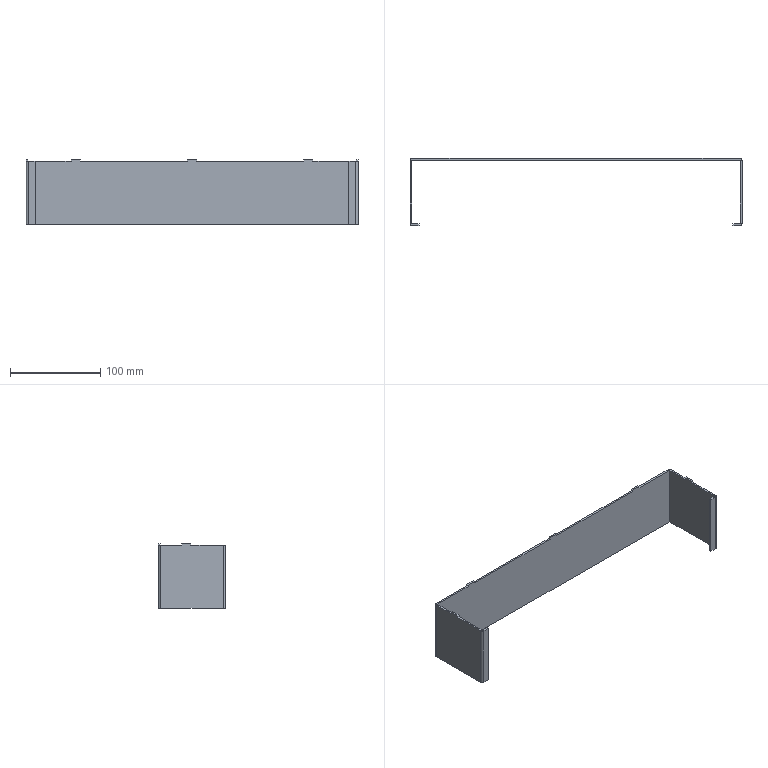Part | STEP file | xzz-004 | 1 solid | 42 faces | box 368 x 74.5 x 72 mm | volume 73899 mm3 | plane 34 | cylinder 8 | commonest cylinder face diameters 1 x4 5 x4
STEP:
#1=CARTESIAN_POINT('',(157.,14.,70.));
#2=VERTEX_POINT('',#1);
#3=CARTESIAN_POINT('',(204.5,14.,70.));
#4=VERTEX_POINT('',#3);
#5=CARTESIAN_POINT('',(-161.,14.,70.));
#6=DIRECTION('',(1.,0.,0.));
#7=VECTOR('',#6,1000.);
#8=LINE('',#5,#7);
#9=EDGE_CURVE('',#2,#4,#8,.T.);
#10=ORIENTED_EDGE('',*,*,#9,.T.);
#11=CARTESIAN_POINT('',(204.5,14.,0.));
#12=VERTEX_POINT('',#11);
#13=CARTESIAN_POINT('',(204.5,14.,70.));
#14=DIRECTION('',(0.,0.,-1.));
#15=VECTOR('',#14,1000.);
#16=LINE('',#13,#15);
#17=EDGE_CURVE('',#4,#12,#16,.T.);
#18=ORIENTED_EDGE('',*,*,#17,.T.);
#19=CARTESIAN_POINT('',(-158.5,14.,0.));
#20=VERTEX_POINT('',#19);
#21=CARTESIAN_POINT('',(-161.,14.,0.));
#22=DIRECTION('',(-1.,0.,0.));
#23=VECTOR('',#22,1000.);
#24=LINE('',#21,#23);
#25=EDGE_CURVE('',#12,#20,#24,.T.);
#26=ORIENTED_EDGE('',*,*,#25,.T.);
#27=CARTESIAN_POINT('',(-158.5,14.,70.));
#28=VERTEX_POINT('',#27);
#29=CARTESIAN_POINT('',(-158.5,14.,70.));
#30=DIRECTION('',(0.,0.,1.));
#31=VECTOR('',#30,1000.);
#32=LINE('',#29,#31);
#33=EDGE_CURVE('',#20,#28,#32,.T.);
#34=ORIENTED_EDGE('',*,*,#33,.T.);
#35=CARTESIAN_POINT('',(-111.,14.,70.));
#36=VERTEX_POINT('',#35);
#37=CARTESIAN_POINT('',(-161.,14.,70.));
#38=DIRECTION('',(1.,0.,0.));
#39=VECTOR('',#38,1000.);
#40=LINE('',#37,#39);
#41=EDGE_CURVE('',#28,#36,#40,.T.);
#42=ORIENTED_EDGE('',*,*,#41,.T.);
#43=CARTESIAN_POINT('',(-111.,14.,72.));
#44=VERTEX_POINT('',#43);
#45=CARTESIAN_POINT('',(-111.,14.,70.));
#46=DIRECTION('',(0.,0.,1.));
#47=VECTOR('',#46,1000.);
#48=LINE('',#45,#47);
#49=EDGE_CURVE('',#36,#44,#48,.T.);
#50=ORIENTED_EDGE('',*,*,#49,.T.);
#51=CARTESIAN_POINT('',(-101.,14.,72.));
#52=VERTEX_POINT('',#51);
#53=CARTESIAN_POINT('',(-161.,14.,72.));
#54=DIRECTION('',(1.,0.,0.));
#55=VECTOR('',#54,1000.);
#56=LINE('',#53,#55);
#57=EDGE_CURVE('',#44,#52,#56,.T.);
#58=ORIENTED_EDGE('',*,*,#57,.T.);
#59=CARTESIAN_POINT('',(-101.,14.,70.));
#60=VERTEX_POINT('',#59);
#61=CARTESIAN_POINT('',(-101.,14.,70.));
#62=DIRECTION('',(0.,0.,-1.));
#63=VECTOR('',#62,1000.);
#64=LINE('',#61,#63);
#65=EDGE_CURVE('',#52,#60,#64,.T.);
#66=ORIENTED_EDGE('',*,*,#65,.T.);
#67=CARTESIAN_POINT('',(18.,14.,70.));
#68=VERTEX_POINT('',#67);
#69=CARTESIAN_POINT('',(-161.,14.,70.));
#70=DIRECTION('',(1.,0.,0.));
#71=VECTOR('',#70,1000.);
#72=LINE('',#69,#71);
#73=EDGE_CURVE('',#60,#68,#72,.T.);
#74=ORIENTED_EDGE('',*,*,#73,.T.);
#75=CARTESIAN_POINT('',(18.,14.,72.));
#76=VERTEX_POINT('',#75);
#77=CARTESIAN_POINT('',(18.,14.,70.));
#78=DIRECTION('',(0.,0.,1.));
#79=VECTOR('',#78,1000.);
#80=LINE('',#77,#79);
#81=EDGE_CURVE('',#68,#76,#80,.T.);
#82=ORIENTED_EDGE('',*,*,#81,.T.);
#83=CARTESIAN_POINT('',(28.,14.,72.));
#84=VERTEX_POINT('',#83);
#85=CARTESIAN_POINT('',(-161.,14.,72.));
#86=DIRECTION('',(1.,0.,0.));
#87=VECTOR('',#86,1000.);
#88=LINE('',#85,#87);
#89=EDGE_CURVE('',#76,#84,#88,.T.);
#90=ORIENTED_EDGE('',*,*,#89,.T.);
#91=CARTESIAN_POINT('',(28.,14.,70.));
#92=VERTEX_POINT('',#91);
#93=CARTESIAN_POINT('',(28.,14.,70.));
#94=DIRECTION('',(0.,0.,-1.));
#95=VECTOR('',#94,1000.);
#96=LINE('',#93,#95);
#97=EDGE_CURVE('',#84,#92,#96,.T.);
#98=ORIENTED_EDGE('',*,*,#97,.T.);
#99=CARTESIAN_POINT('',(147.,14.,70.));
#100=VERTEX_POINT('',#99);
#101=CARTESIAN_POINT('',(-161.,14.,70.));
#102=DIRECTION('',(1.,0.,0.));
#103=VECTOR('',#102,1000.);
#104=LINE('',#101,#103);
#105=EDGE_CURVE('',#92,#100,#104,.T.);
#106=ORIENTED_EDGE('',*,*,#105,.T.);
#107=CARTESIAN_POINT('',(147.,14.,72.));
#108=VERTEX_POINT('',#107);
#109=CARTESIAN_POINT('',(147.,14.,70.));
#110=DIRECTION('',(0.,0.,1.));
#111=VECTOR('',#110,1000.);
#112=LINE('',#109,#111);
#113=EDGE_CURVE('',#100,#108,#112,.T.);
#114=ORIENTED_EDGE('',*,*,#113,.T.);
#115=CARTESIAN_POINT('',(157.,14.,72.));
#116=VERTEX_POINT('',#115);
#117=CARTESIAN_POINT('',(-161.,14.,72.));
#118=DIRECTION('',(1.,0.,0.));
#119=VECTOR('',#118,1000.);
#120=LINE('',#117,#119);
#121=EDGE_CURVE('',#108,#116,#120,.T.);
#122=ORIENTED_EDGE('',*,*,#121,.T.);
#123=CARTESIAN_POINT('',(157.,14.,70.));
#124=DIRECTION('',(0.,0.,-1.));
#125=VECTOR('',#124,1000.);
#126=LINE('',#123,#125);
#127=EDGE_CURVE('',#116,#2,#126,.T.);
#128=ORIENTED_EDGE('',*,*,#127,.T.);
#129=EDGE_LOOP('',(#10,#18,#26,#34,#42,#50,#58,#66,#74,#82,#90,#98,#106,#114,#122,#128));
#130=FACE_OUTER_BOUND('',#129,.T.);
#131=CARTESIAN_POINT('',(-161.,14.,70.));
#132=DIRECTION('',(0.,1.,0.));
#133=DIRECTION('',(0.,0.,1.));
#134=AXIS2_PLACEMENT_3D('',#131,#132,#133);
#135=PLANE('',#134);
#136=ADVANCED_FACE('',(#130),#135,.T.);
#137=CARTESIAN_POINT('',(207.,11.5,70.));
#138=VERTEX_POINT('',#137);
#139=CARTESIAN_POINT('',(204.5,11.5,70.));
#140=DIRECTION('',(0.,0.,-1.));
#141=DIRECTION('',(-1.,0.,0.));
#142=AXIS2_PLACEMENT_3D('',#139,#140,#141);
#143=CIRCLE('',#142,2.5);
#144=EDGE_CURVE('',#4,#138,#143,.T.);
#145=ORIENTED_EDGE('',*,*,#144,.T.);
#146=CARTESIAN_POINT('',(207.,11.5,0.));
#147=VERTEX_POINT('',#146);
#148=CARTESIAN_POINT('',(207.,11.5,70.));
#149=DIRECTION('',(0.,0.,-1.));
#150=VECTOR('',#149,1000.);
#151=LINE('',#148,#150);
#152=EDGE_CURVE('',#138,#147,#151,.T.);
#153=ORIENTED_EDGE('',*,*,#152,.T.);
#154=CARTESIAN_POINT('',(204.5,11.5,0.));
#155=DIRECTION('',(0.,0.,1.));
#156=DIRECTION('',(-1.,0.,0.));
#157=AXIS2_PLACEMENT_3D('',#154,#155,#156);
#158=CIRCLE('',#157,2.5);
#159=EDGE_CURVE('',#147,#12,#158,.T.);
#160=ORIENTED_EDGE('',*,*,#159,.T.);
#161=ORIENTED_EDGE('',*,*,#17,.F.);
#162=EDGE_LOOP('',(#145,#153,#160,#161));
#163=FACE_OUTER_BOUND('',#162,.T.);
#164=CARTESIAN_POINT('',(204.5,11.5,70.));
#165=DIRECTION('',(0.,0.,-1.));
#166=DIRECTION('',(-1.,0.,0.));
#167=AXIS2_PLACEMENT_3D('',#164,#165,#166);
#168=CYLINDRICAL_SURFACE('',#167,2.5);
#169=ADVANCED_FACE('',(#163),#168,.T.);
#170=CARTESIAN_POINT('',(157.,12.,70.));
#171=VERTEX_POINT('',#170);
#172=CARTESIAN_POINT('',(204.5,12.,70.));
#173=VERTEX_POINT('',#172);
#174=CARTESIAN_POINT('',(-159.,12.,70.));
#175=DIRECTION('',(1.,0.,0.));
#176=VECTOR('',#175,1000.);
#177=LINE('',#174,#176);
#178=EDGE_CURVE('',#171,#173,#177,.T.);
#179=ORIENTED_EDGE('',*,*,#178,.T.);
#180=CARTESIAN_POINT('',(205.,11.5,70.));
#181=VERTEX_POINT('',#180);
#182=CARTESIAN_POINT('',(204.5,11.5,70.));
#183=DIRECTION('',(0.,0.,-1.));
#184=DIRECTION('',(-1.,0.,0.));
#185=AXIS2_PLACEMENT_3D('',#182,#183,#184);
#186=CIRCLE('',#185,0.5);
#187=EDGE_CURVE('',#173,#181,#186,.T.);
#188=ORIENTED_EDGE('',*,*,#187,.T.);
#189=CARTESIAN_POINT('',(205.,-12.,70.));
#190=VERTEX_POINT('',#189);
#191=CARTESIAN_POINT('',(205.,12.,70.));
#192=DIRECTION('',(0.,-1.,0.));
#193=VECTOR('',#192,1000.);
#194=LINE('',#191,#193);
#195=EDGE_CURVE('',#181,#190,#194,.T.);
#196=ORIENTED_EDGE('',*,*,#195,.T.);
#197=CARTESIAN_POINT('',(207.,-12.,70.));
#198=VERTEX_POINT('',#197);
#199=CARTESIAN_POINT('',(205.,-12.,70.));
#200=DIRECTION('',(1.,0.,0.));
#201=VECTOR('',#200,1000.);
#202=LINE('',#199,#201);
#203=EDGE_CURVE('',#190,#198,#202,.T.);
#204=ORIENTED_EDGE('',*,*,#203,.T.);
#205=CARTESIAN_POINT('',(207.,14.,70.));
#206=DIRECTION('',(0.,-1.,0.));
#207=VECTOR('',#206,1000.);
#208=LINE('',#205,#207);
#209=EDGE_CURVE('',#138,#198,#208,.T.);
#210=ORIENTED_EDGE('',*,*,#209,.F.);
#211=ORIENTED_EDGE('',*,*,#144,.F.);
#212=ORIENTED_EDGE('',*,*,#9,.F.);
#213=CARTESIAN_POINT('',(157.,11.5,70.));
#214=DIRECTION('',(0.,-1.,0.));
#215=VECTOR('',#214,1000.);
#216=LINE('',#213,#215);
#217=EDGE_CURVE('',#2,#171,#216,.T.);
#218=ORIENTED_EDGE('',*,*,#217,.T.);
#219=EDGE_LOOP('',(#179,#188,#196,#204,#210,#211,#212,#218));
#220=FACE_OUTER_BOUND('',#219,.T.);
#221=CARTESIAN_POINT('',(-159.,11.5,70.));
#222=DIRECTION('',(0.,0.,1.));
#223=DIRECTION('',(1.,0.,0.));
#224=AXIS2_PLACEMENT_3D('',#221,#222,#223);
#225=PLANE('',#224);
#226=ADVANCED_FACE('',(#220),#225,.T.);
#227=ORIENTED_EDGE('',*,*,#127,.F.);
#228=CARTESIAN_POINT('',(157.,12.,72.));
#229=VERTEX_POINT('',#228);
#230=CARTESIAN_POINT('',(157.,14.,72.));
#231=DIRECTION('',(0.,1.,0.));
#232=VECTOR('',#231,1000.);
#233=LINE('',#230,#232);
#234=EDGE_CURVE('',#229,#116,#233,.T.);
#235=ORIENTED_EDGE('',*,*,#234,.F.);
#236=CARTESIAN_POINT('',(157.,12.,72.));
#237=DIRECTION('',(0.,0.,1.));
#238=VECTOR('',#237,1000.);
#239=LINE('',#236,#238);
#240=EDGE_CURVE('',#171,#229,#239,.T.);
#241=ORIENTED_EDGE('',*,*,#240,.F.);
#242=ORIENTED_EDGE('',*,*,#217,.F.);
#243=EDGE_LOOP('',(#227,#235,#241,#242));
#244=FACE_OUTER_BOUND('',#243,.T.);
#245=CARTESIAN_POINT('',(157.,14.,72.));
#246=DIRECTION('',(-1.,0.,0.));
#247=DIRECTION('',(0.,0.,1.));
#248=AXIS2_PLACEMENT_3D('',#245,#246,#247);
#249=PLANE('',#248);
#250=ADVANCED_FACE('',(#244),#249,.F.);
#251=ORIENTED_EDGE('',*,*,#234,.T.);
#252=ORIENTED_EDGE('',*,*,#121,.F.);
#253=CARTESIAN_POINT('',(147.,12.,72.));
#254=VERTEX_POINT('',#253);
#255=CARTESIAN_POINT('',(147.,0.,72.));
#256=DIRECTION('',(0.,-1.,0.));
#257=VECTOR('',#256,1000.);
#258=LINE('',#255,#257);
#259=EDGE_CURVE('',#108,#254,#258,.T.);
#260=ORIENTED_EDGE('',*,*,#259,.T.);
#261=CARTESIAN_POINT('',(0.,12.,72.));
#262=DIRECTION('',(1.,0.,0.));
#263=VECTOR('',#262,1000.);
#264=LINE('',#261,#263);
#265=EDGE_CURVE('',#254,#229,#264,.T.);
#266=ORIENTED_EDGE('',*,*,#265,.T.);
#267=EDGE_LOOP('',(#251,#252,#260,#266));
#268=FACE_OUTER_BOUND('',#267,.T.);
#269=CARTESIAN_POINT('',(0.,0.,72.));
#270=DIRECTION('',(0.,0.,1.));
#271=DIRECTION('',(1.,0.,0.));
#272=AXIS2_PLACEMENT_3D('',#269,#270,#271);
#273=PLANE('',#272);
#274=ADVANCED_FACE('',(#268),#273,.T.);
#275=CARTESIAN_POINT('',(147.,12.,70.));
#276=VERTEX_POINT('',#275);
#277=CARTESIAN_POINT('',(147.,12.,72.));
#278=DIRECTION('',(0.,0.,-1.));
#279=VECTOR('',#278,1000.);
#280=LINE('',#277,#279);
#281=EDGE_CURVE('',#254,#276,#280,.T.);
#282=ORIENTED_EDGE('',*,*,#281,.F.);
#283=ORIENTED_EDGE('',*,*,#259,.F.);
#284=ORIENTED_EDGE('',*,*,#113,.F.);
#285=CARTESIAN_POINT('',(147.,14.,70.));
#286=DIRECTION('',(0.,1.,0.));
#287=VECTOR('',#286,1000.);
#288=LINE('',#285,#287);
#289=EDGE_CURVE('',#276,#100,#288,.T.);
#290=ORIENTED_EDGE('',*,*,#289,.F.);
#291=EDGE_LOOP('',(#282,#283,#284,#290));
#292=FACE_OUTER_BOUND('',#291,.T.);
#293=CARTESIAN_POINT('',(147.,14.,72.));
#294=DIRECTION('',(1.,0.,0.));
#295=DIRECTION('',(0.,0.,-1.));
#296=AXIS2_PLACEMENT_3D('',#293,#294,#295);
#297=PLANE('',#296);
#298=ADVANCED_FACE('',(#292),#297,.F.);
#299=ORIENTED_EDGE('',*,*,#105,.F.);
#300=CARTESIAN_POINT('',(28.,12.,70.));
#301=VERTEX_POINT('',#300);
#302=CARTESIAN_POINT('',(28.,11.5,70.));
#303=DIRECTION('',(0.,-1.,0.));
#304=VECTOR('',#303,1000.);
#305=LINE('',#302,#304);
#306=EDGE_CURVE('',#92,#301,#305,.T.);
#307=ORIENTED_EDGE('',*,*,#306,.T.);
#308=CARTESIAN_POINT('',(-159.,12.,70.));
#309=DIRECTION('',(1.,0.,0.));
#310=VECTOR('',#309,1000.);
#311=LINE('',#308,#310);
#312=EDGE_CURVE('',#301,#276,#311,.T.);
#313=ORIENTED_EDGE('',*,*,#312,.T.);
#314=ORIENTED_EDGE('',*,*,#289,.T.);
#315=EDGE_LOOP('',(#299,#307,#313,#314));
#316=FACE_OUTER_BOUND('',#315,.T.);
#317=CARTESIAN_POINT('',(-159.,11.5,70.));
#318=DIRECTION('',(0.,0.,1.));
#319=DIRECTION('',(1.,0.,0.));
#320=AXIS2_PLACEMENT_3D('',#317,#318,#319);
#321=PLANE('',#320);
#322=ADVANCED_FACE('',(#316),#321,.T.);
#323=ORIENTED_EDGE('',*,*,#97,.F.);
#324=CARTESIAN_POINT('',(28.,12.,72.));
#325=VERTEX_POINT('',#324);
#326=CARTESIAN_POINT('',(28.,14.,72.));
#327=DIRECTION('',(0.,1.,0.));
#328=VECTOR('',#327,1000.);
#329=LINE('',#326,#328);
#330=EDGE_CURVE('',#325,#84,#329,.T.);
#331=ORIENTED_EDGE('',*,*,#330,.F.);
#332=CARTESIAN_POINT('',(28.,12.,72.));
#333=DIRECTION('',(0.,0.,1.));
#334=VECTOR('',#333,1000.);
#335=LINE('',#332,#334);
#336=EDGE_CURVE('',#301,#325,#335,.T.);
#337=ORIENTED_EDGE('',*,*,#336,.F.);
#338=ORIENTED_EDGE('',*,*,#306,.F.);
#339=EDGE_LOOP('',(#323,#331,#337,#338));
#340=FACE_OUTER_BOUND('',#339,.T.);
#341=CARTESIAN_POINT('',(28.,14.,72.));
#342=DIRECTION('',(-1.,0.,0.));
#343=DIRECTION('',(0.,0.,1.));
#344=AXIS2_PLACEMENT_3D('',#341,#342,#343);
#345=PLANE('',#344);
#346=ADVANCED_FACE('',(#340),#345,.F.);
#347=ORIENTED_EDGE('',*,*,#330,.T.);
#348=ORIENTED_EDGE('',*,*,#89,.F.);
#349=CARTESIAN_POINT('',(18.,12.,72.));
#350=VERTEX_POINT('',#349);
#351=CARTESIAN_POINT('',(18.,0.,72.));
#352=DIRECTION('',(0.,-1.,0.));
#353=VECTOR('',#352,1000.);
#354=LINE('',#351,#353);
#355=EDGE_CURVE('',#76,#350,#354,.T.);
#356=ORIENTED_EDGE('',*,*,#355,.T.);
#357=CARTESIAN_POINT('',(0.,12.,72.));
#358=DIRECTION('',(1.,0.,0.));
#359=VECTOR('',#358,1000.);
#360=LINE('',#357,#359);
#361=EDGE_CURVE('',#350,#325,#360,.T.);
#362=ORIENTED_EDGE('',*,*,#361,.T.);
#363=EDGE_LOOP('',(#347,#348,#356,#362));
#364=FACE_OUTER_BOUND('',#363,.T.);
#365=CARTESIAN_POINT('',(0.,0.,72.));
#366=DIRECTION('',(0.,0.,1.));
#367=DIRECTION('',(1.,0.,0.));
#368=AXIS2_PLACEMENT_3D('',#365,#366,#367);
#369=PLANE('',#368);
#370=ADVANCED_FACE('',(#364),#369,.T.);
#371=CARTESIAN_POINT('',(18.,12.,70.));
#372=VERTEX_POINT('',#371);
#373=CARTESIAN_POINT('',(18.,12.,72.));
#374=DIRECTION('',(0.,0.,-1.));
#375=VECTOR('',#374,1000.);
#376=LINE('',#373,#375);
#377=EDGE_CURVE('',#350,#372,#376,.T.);
#378=ORIENTED_EDGE('',*,*,#377,.F.);
#379=ORIENTED_EDGE('',*,*,#355,.F.);
#380=ORIENTED_EDGE('',*,*,#81,.F.);
#381=CARTESIAN_POINT('',(18.,14.,70.));
#382=DIRECTION('',(0.,1.,0.));
#383=VECTOR('',#382,1000.);
#384=LINE('',#381,#383);
#385=EDGE_CURVE('',#372,#68,#384,.T.);
#386=ORIENTED_EDGE('',*,*,#385,.F.);
#387=EDGE_LOOP('',(#378,#379,#380,#386));
#388=FACE_OUTER_BOUND('',#387,.T.);
#389=CARTESIAN_POINT('',(18.,14.,72.));
#390=DIRECTION('',(1.,0.,0.));
#391=DIRECTION('',(0.,0.,-1.));
#392=AXIS2_PLACEMENT_3D('',#389,#390,#391);
#393=PLANE('',#392);
#394=ADVANCED_FACE('',(#388),#393,.F.);
#395=ORIENTED_EDGE('',*,*,#73,.F.);
#396=CARTESIAN_POINT('',(-101.,12.,70.));
#397=VERTEX_POINT('',#396);
#398=CARTESIAN_POINT('',(-101.,11.5,70.));
#399=DIRECTION('',(0.,-1.,0.));
#400=VECTOR('',#399,1000.);
#401=LINE('',#398,#400);
#402=EDGE_CURVE('',#60,#397,#401,.T.);
#403=ORIENTED_EDGE('',*,*,#402,.T.);
#404=CARTESIAN_POINT('',(-159.,12.,70.));
#405=DIRECTION('',(1.,0.,0.));
#406=VECTOR('',#405,1000.);
#407=LINE('',#404,#406);
#408=EDGE_CURVE('',#397,#372,#407,.T.);
#409=ORIENTED_EDGE('',*,*,#408,.T.);
#410=ORIENTED_EDGE('',*,*,#385,.T.);
#411=EDGE_LOOP('',(#395,#403,#409,#410));
#412=FACE_OUTER_BOUND('',#411,.T.);
#413=CARTESIAN_POINT('',(-159.,11.5,70.));
#414=DIRECTION('',(0.,0.,1.));
#415=DIRECTION('',(1.,0.,0.));
#416=AXIS2_PLACEMENT_3D('',#413,#414,#415);
#417=PLANE('',#416);
#418=ADVANCED_FACE('',(#412),#417,.T.);
#419=ORIENTED_EDGE('',*,*,#65,.F.);
#420=CARTESIAN_POINT('',(-101.,12.,72.));
#421=VERTEX_POINT('',#420);
#422=CARTESIAN_POINT('',(-101.,14.,72.));
#423=DIRECTION('',(0.,1.,0.));
#424=VECTOR('',#423,1000.);
#425=LINE('',#422,#424);
#426=EDGE_CURVE('',#421,#52,#425,.T.);
#427=ORIENTED_EDGE('',*,*,#426,.F.);
#428=CARTESIAN_POINT('',(-101.,12.,72.));
#429=DIRECTION('',(0.,0.,1.));
#430=VECTOR('',#429,1000.);
#431=LINE('',#428,#430);
#432=EDGE_CURVE('',#397,#421,#431,.T.);
#433=ORIENTED_EDGE('',*,*,#432,.F.);
#434=ORIENTED_EDGE('',*,*,#402,.F.);
#435=EDGE_LOOP('',(#419,#427,#433,#434));
#436=FACE_OUTER_BOUND('',#435,.T.);
#437=CARTESIAN_POINT('',(-101.,14.,72.));
#438=DIRECTION('',(-1.,0.,0.));
#439=DIRECTION('',(0.,0.,1.));
#440=AXIS2_PLACEMENT_3D('',#437,#438,#439);
#441=PLANE('',#440);
#442=ADVANCED_FACE('',(#436),#441,.F.);
#443=ORIENTED_EDGE('',*,*,#426,.T.);
#444=ORIENTED_EDGE('',*,*,#57,.F.);
#445=CARTESIAN_POINT('',(-111.,12.,72.));
#446=VERTEX_POINT('',#445);
#447=CARTESIAN_POINT('',(-111.,0.,72.));
#448=DIRECTION('',(0.,-1.,0.));
#449=VECTOR('',#448,1000.);
#450=LINE('',#447,#449);
#451=EDGE_CURVE('',#44,#446,#450,.T.);
#452=ORIENTED_EDGE('',*,*,#451,.T.);
#453=CARTESIAN_POINT('',(0.,12.,72.));
#454=DIRECTION('',(1.,0.,0.));
#455=VECTOR('',#454,1000.);
#456=LINE('',#453,#455);
#457=EDGE_CURVE('',#446,#421,#456,.T.);
#458=ORIENTED_EDGE('',*,*,#457,.T.);
#459=EDGE_LOOP('',(#443,#444,#452,#458));
#460=FACE_OUTER_BOUND('',#459,.T.);
#461=CARTESIAN_POINT('',(0.,0.,72.));
#462=DIRECTION('',(0.,0.,1.));
#463=DIRECTION('',(1.,0.,0.));
#464=AXIS2_PLACEMENT_3D('',#461,#462,#463);
#465=PLANE('',#464);
#466=ADVANCED_FACE('',(#460),#465,.T.);
#467=CARTESIAN_POINT('',(-111.,12.,70.));
#468=VERTEX_POINT('',#467);
#469=CARTESIAN_POINT('',(-111.,12.,72.));
#470=DIRECTION('',(0.,0.,-1.));
#471=VECTOR('',#470,1000.);
#472=LINE('',#469,#471);
#473=EDGE_CURVE('',#446,#468,#472,.T.);
#474=ORIENTED_EDGE('',*,*,#473,.F.);
#475=ORIENTED_EDGE('',*,*,#451,.F.);
#476=ORIENTED_EDGE('',*,*,#49,.F.);
#477=CARTESIAN_POINT('',(-111.,14.,70.));
#478=DIRECTION('',(0.,1.,0.));
#479=VECTOR('',#478,1000.);
#480=LINE('',#477,#479);
#481=EDGE_CURVE('',#468,#36,#480,.T.);
#482=ORIENTED_EDGE('',*,*,#481,.F.);
#483=EDGE_LOOP('',(#474,#475,#476,#482));
#484=FACE_OUTER_BOUND('',#483,.T.);
#485=CARTESIAN_POINT('',(-111.,14.,72.));
#486=DIRECTION('',(1.,0.,0.));
#487=DIRECTION('',(0.,0.,-1.));
#488=AXIS2_PLACEMENT_3D('',#485,#486,#487);
#489=PLANE('',#488);
#490=ADVANCED_FACE('',(#484),#489,.F.);
#491=ORIENTED_EDGE('',*,*,#41,.F.);
#492=CARTESIAN_POINT('',(-161.,11.5,70.));
#493=VERTEX_POINT('',#492);
#494=CARTESIAN_POINT('',(-158.5,11.5,70.));
#495=DIRECTION('',(0.,0.,-1.));
#496=DIRECTION('',(-1.,0.,0.));
#497=AXIS2_PLACEMENT_3D('',#494,#495,#496);
#498=CIRCLE('',#497,2.5);
#499=EDGE_CURVE('',#493,#28,#498,.T.);
#500=ORIENTED_EDGE('',*,*,#499,.F.);
#501=CARTESIAN_POINT('',(-161.,-12.,70.));
#502=VERTEX_POINT('',#501);
#503=CARTESIAN_POINT('',(-161.,14.,70.));
#504=DIRECTION('',(0.,1.,0.));
#505=VECTOR('',#504,1000.);
#506=LINE('',#503,#505);
#507=EDGE_CURVE('',#502,#493,#506,.T.);
#508=ORIENTED_EDGE('',*,*,#507,.F.);
#509=CARTESIAN_POINT('',(-159.,-12.,70.));
#510=VERTEX_POINT('',#509);
#511=CARTESIAN_POINT('',(-158.5,-12.,70.));
#512=DIRECTION('',(1.,0.,0.));
#513=VECTOR('',#512,1000.);
#514=LINE('',#511,#513);
#515=EDGE_CURVE('',#502,#510,#514,.T.);
#516=ORIENTED_EDGE('',*,*,#515,.T.);
#517=CARTESIAN_POINT('',(-159.,11.5,70.));
#518=VERTEX_POINT('',#517);
#519=CARTESIAN_POINT('',(-159.,-58.5,70.));
#520=DIRECTION('',(0.,1.,0.));
#521=VECTOR('',#520,1000.);
#522=LINE('',#519,#521);
#523=EDGE_CURVE('',#510,#518,#522,.T.);
#524=ORIENTED_EDGE('',*,*,#523,.T.);
#525=CARTESIAN_POINT('',(-158.5,12.,70.));
#526=VERTEX_POINT('',#525);
#527=CARTESIAN_POINT('',(-158.5,11.5,70.));
#528=DIRECTION('',(0.,0.,-1.));
#529=DIRECTION('',(-1.,0.,0.));
#530=AXIS2_PLACEMENT_3D('',#527,#528,#529);
#531=CIRCLE('',#530,0.5);
#532=EDGE_CURVE('',#518,#526,#531,.T.);
#533=ORIENTED_EDGE('',*,*,#532,.T.);
#534=CARTESIAN_POINT('',(-159.,12.,70.));
#535=DIRECTION('',(1.,0.,0.));
#536=VECTOR('',#535,1000.);
#537=LINE('',#534,#536);
#538=EDGE_CURVE('',#526,#468,#537,.T.);
#539=ORIENTED_EDGE('',*,*,#538,.T.);
#540=ORIENTED_EDGE('',*,*,#481,.T.);
#541=EDGE_LOOP('',(#491,#500,#508,#516,#524,#533,#539,#540));
#542=FACE_OUTER_BOUND('',#541,.T.);
#543=CARTESIAN_POINT('',(-159.,11.5,70.));
#544=DIRECTION('',(0.,0.,1.));
#545=DIRECTION('',(1.,0.,0.));
#546=AXIS2_PLACEMENT_3D('',#543,#544,#545);
#547=PLANE('',#546);
#548=ADVANCED_FACE('',(#542),#547,.T.);
#549=ORIENTED_EDGE('',*,*,#499,.T.);
#550=ORIENTED_EDGE('',*,*,#33,.F.);
#551=CARTESIAN_POINT('',(-161.,11.5,0.));
#552=VERTEX_POINT('',#551);
#553=CARTESIAN_POINT('',(-158.5,11.5,0.));
#554=DIRECTION('',(0.,0.,1.));
#555=DIRECTION('',(-1.,0.,0.));
#556=AXIS2_PLACEMENT_3D('',#553,#554,#555);
#557=CIRCLE('',#556,2.5);
#558=EDGE_CURVE('',#20,#552,#557,.T.);
#559=ORIENTED_EDGE('',*,*,#558,.T.);
#560=CARTESIAN_POINT('',(-161.,11.5,70.));
#561=DIRECTION('',(0.,0.,1.));
#562=VECTOR('',#561,1000.);
#563=LINE('',#560,#562);
#564=EDGE_CURVE('',#552,#493,#563,.T.);
#565=ORIENTED_EDGE('',*,*,#564,.T.);
#566=EDGE_LOOP('',(#549,#550,#559,#565));
#567=FACE_OUTER_BOUND('',#566,.T.);
#568=CARTESIAN_POINT('',(-158.5,11.5,70.));
#569=DIRECTION('',(0.,0.,-1.));
#570=DIRECTION('',(-1.,0.,0.));
#571=AXIS2_PLACEMENT_3D('',#568,#569,#570);
#572=CYLINDRICAL_SURFACE('',#571,2.5);
#573=ADVANCED_FACE('',(#567),#572,.T.);
#574=CARTESIAN_POINT('',(204.5,12.,0.));
#575=VERTEX_POINT('',#574);
#576=CARTESIAN_POINT('',(-158.5,12.,0.));
#577=VERTEX_POINT('',#576);
#578=CARTESIAN_POINT('',(205.,12.,0.));
#579=DIRECTION('',(-1.,0.,0.));
#580=VECTOR('',#579,1000.);
#581=LINE('',#578,#580);
#582=EDGE_CURVE('',#575,#577,#581,.T.);
#583=ORIENTED_EDGE('',*,*,#582,.T.);
#584=CARTESIAN_POINT('',(-159.,11.5,0.));
#585=VERTEX_POINT('',#584);
#586=CARTESIAN_POINT('',(-158.5,11.5,0.));
#587=DIRECTION('',(0.,0.,1.));
#588=DIRECTION('',(-1.,0.,0.));
#589=AXIS2_PLACEMENT_3D('',#586,#587,#588);
#590=CIRCLE('',#589,0.5);
#591=EDGE_CURVE('',#577,#585,#590,.T.);
#592=ORIENTED_EDGE('',*,*,#591,.T.);
#593=CARTESIAN_POINT('',(-159.,-58.,0.));
#594=VERTEX_POINT('',#593);
#595=CARTESIAN_POINT('',(-159.,12.,0.));
#596=DIRECTION('',(0.,-1.,0.));
#597=VECTOR('',#596,1000.);
#598=LINE('',#595,#597);
#599=EDGE_CURVE('',#585,#594,#598,.T.);
#600=ORIENTED_EDGE('',*,*,#599,.T.);
#601=CARTESIAN_POINT('',(-158.5,-58.5,0.));
#602=VERTEX_POINT('',#601);
#603=CARTESIAN_POINT('',(-158.5,-58.,0.));
#604=DIRECTION('',(0.,0.,1.));
#605=DIRECTION('',(-1.,0.,0.));
#606=AXIS2_PLACEMENT_3D('',#603,#604,#605);
#607=CIRCLE('',#606,0.5);
#608=EDGE_CURVE('',#594,#602,#607,.T.);
#609=ORIENTED_EDGE('',*,*,#608,.T.);
#610=CARTESIAN_POINT('',(-151.,-58.5,0.));
#611=VERTEX_POINT('',#610);
#612=CARTESIAN_POINT('',(-159.,-58.5,0.));
#613=DIRECTION('',(1.,0.,0.));
#614=VECTOR('',#613,1000.);
#615=LINE('',#612,#614);
#616=EDGE_CURVE('',#602,#611,#615,.T.);
#617=ORIENTED_EDGE('',*,*,#616,.T.);
#618=CARTESIAN_POINT('',(-151.,-60.5,0.));
#619=VERTEX_POINT('',#618);
#620=CARTESIAN_POINT('',(-151.,-58.5,0.));
#621=DIRECTION('',(0.,1.,0.));
#622=VECTOR('',#621,1000.);
#623=LINE('',#620,#622);
#624=EDGE_CURVE('',#619,#611,#623,.T.);
#625=ORIENTED_EDGE('',*,*,#624,.F.);
#626=CARTESIAN_POINT('',(-158.5,-60.5,0.));
#627=VERTEX_POINT('',#626);
#628=CARTESIAN_POINT('',(-161.,-60.5,0.));
#629=DIRECTION('',(1.,0.,0.));
#630=VECTOR('',#629,1000.);
#631=LINE('',#628,#630);
#632=EDGE_CURVE('',#627,#619,#631,.T.);
#633=ORIENTED_EDGE('',*,*,#632,.F.);
#634=CARTESIAN_POINT('',(-161.,-58.,0.));
#635=VERTEX_POINT('',#634);
#636=CARTESIAN_POINT('',(-158.5,-58.,0.));
#637=DIRECTION('',(0.,0.,1.));
#638=DIRECTION('',(-1.,0.,0.));
#639=AXIS2_PLACEMENT_3D('',#636,#637,#638);
#640=CIRCLE('',#639,2.5);
#641=EDGE_CURVE('',#635,#627,#640,.T.);
#642=ORIENTED_EDGE('',*,*,#641,.F.);
#643=CARTESIAN_POINT('',(-161.,14.,0.));
#644=DIRECTION('',(0.,-1.,0.));
#645=VECTOR('',#644,1000.);
#646=LINE('',#643,#645);
#647=EDGE_CURVE('',#552,#635,#646,.T.);
#648=ORIENTED_EDGE('',*,*,#647,.F.);
#649=ORIENTED_EDGE('',*,*,#558,.F.);
#650=ORIENTED_EDGE('',*,*,#25,.F.);
#651=ORIENTED_EDGE('',*,*,#159,.F.);
#652=CARTESIAN_POINT('',(207.,-58.,0.));
#653=VERTEX_POINT('',#652);
#654=CARTESIAN_POINT('',(207.,14.,0.));
#655=DIRECTION('',(0.,1.,0.));
#656=VECTOR('',#655,1000.);
#657=LINE('',#654,#656);
#658=EDGE_CURVE('',#653,#147,#657,.T.);
#659=ORIENTED_EDGE('',*,*,#658,.F.);
#660=CARTESIAN_POINT('',(204.5,-60.5,0.));
#661=VERTEX_POINT('',#660);
#662=CARTESIAN_POINT('',(204.5,-58.,0.));
#663=DIRECTION('',(0.,0.,1.));
#664=DIRECTION('',(-1.,0.,0.));
#665=AXIS2_PLACEMENT_3D('',#662,#663,#664);
#666=CIRCLE('',#665,2.5);
#667=EDGE_CURVE('',#661,#653,#666,.T.);
#668=ORIENTED_EDGE('',*,*,#667,.F.);
#669=CARTESIAN_POINT('',(197.,-60.5,0.));
#670=VERTEX_POINT('',#669);
#671=CARTESIAN_POINT('',(207.,-60.5,0.));
#672=DIRECTION('',(1.,0.,0.));
#673=VECTOR('',#672,1000.);
#674=LINE('',#671,#673);
#675=EDGE_CURVE('',#670,#661,#674,.T.);
#676=ORIENTED_EDGE('',*,*,#675,.F.);
#677=CARTESIAN_POINT('',(197.,-58.5,0.));
#678=VERTEX_POINT('',#677);
#679=CARTESIAN_POINT('',(197.,-60.5,0.));
#680=DIRECTION('',(0.,-1.,0.));
#681=VECTOR('',#680,1000.);
#682=LINE('',#679,#681);
#683=EDGE_CURVE('',#678,#670,#682,.T.);
#684=ORIENTED_EDGE('',*,*,#683,.F.);
#685=CARTESIAN_POINT('',(204.5,-58.5,0.));
#686=VERTEX_POINT('',#685);
#687=CARTESIAN_POINT('',(204.5,-58.5,0.));
#688=DIRECTION('',(-1.,0.,0.));
#689=VECTOR('',#688,1000.);
#690=LINE('',#687,#689);
#691=EDGE_CURVE('',#686,#678,#690,.T.);
#692=ORIENTED_EDGE('',*,*,#691,.F.);
#693=CARTESIAN_POINT('',(205.,-58.,0.));
#694=VERTEX_POINT('',#693);
#695=CARTESIAN_POINT('',(204.5,-58.,0.));
#696=DIRECTION('',(0.,0.,1.));
#697=DIRECTION('',(-1.,0.,0.));
#698=AXIS2_PLACEMENT_3D('',#695,#696,#697);
#699=CIRCLE('',#698,0.5);
#700=EDGE_CURVE('',#686,#694,#699,.T.);
#701=ORIENTED_EDGE('',*,*,#700,.T.);
#702=CARTESIAN_POINT('',(205.,11.5,0.));
#703=VERTEX_POINT('',#702);
#704=CARTESIAN_POINT('',(205.,-58.5,0.));
#705=DIRECTION('',(0.,1.,0.));
#706=VECTOR('',#705,1000.);
#707=LINE('',#704,#706);
#708=EDGE_CURVE('',#694,#703,#707,.T.);
#709=ORIENTED_EDGE('',*,*,#708,.T.);
#710=CARTESIAN_POINT('',(204.5,11.5,0.));
#711=DIRECTION('',(0.,0.,1.));
#712=DIRECTION('',(-1.,0.,0.));
#713=AXIS2_PLACEMENT_3D('',#710,#711,#712);
#714=CIRCLE('',#713,0.5);
#715=EDGE_CURVE('',#703,#575,#714,.T.);
#716=ORIENTED_EDGE('',*,*,#715,.T.);
#717=EDGE_LOOP('',(#583,#592,#600,#609,#617,#625,#633,#642,#648,#649,#650,#651,#659,#668,#676,#684,#692,#701,#709,#716));
#718=FACE_OUTER_BOUND('',#717,.T.);
#719=CARTESIAN_POINT('',(205.,11.5,0.));
#720=DIRECTION('',(0.,0.,-1.));
#721=DIRECTION('',(-1.,0.,0.));
#722=AXIS2_PLACEMENT_3D('',#719,#720,#721);
#723=PLANE('',#722);
#724=ADVANCED_FACE('',(#718),#723,.T.);
#725=CARTESIAN_POINT('',(207.,-22.,70.));
#726=VERTEX_POINT('',#725);
#727=CARTESIAN_POINT('',(207.,-58.,70.));
#728=VERTEX_POINT('',#727);
#729=CARTESIAN_POINT('',(207.,14.,70.));
#730=DIRECTION('',(0.,-1.,0.));
#731=VECTOR('',#730,1000.);
#732=LINE('',#729,#731);
#733=EDGE_CURVE('',#726,#728,#732,.T.);
#734=ORIENTED_EDGE('',*,*,#733,.T.);
#735=CARTESIAN_POINT('',(207.,-58.,70.));
#736=DIRECTION('',(0.,0.,-1.));
#737=VECTOR('',#736,1000.);
#738=LINE('',#735,#737);
#739=EDGE_CURVE('',#728,#653,#738,.T.);
#740=ORIENTED_EDGE('',*,*,#739,.T.);
#741=ORIENTED_EDGE('',*,*,#658,.T.);
#742=ORIENTED_EDGE('',*,*,#152,.F.);
#743=ORIENTED_EDGE('',*,*,#209,.T.);
#744=CARTESIAN_POINT('',(207.,-12.,72.));
#745=VERTEX_POINT('',#744);
#746=CARTESIAN_POINT('',(207.,-12.,70.));
#747=DIRECTION('',(0.,0.,1.));
#748=VECTOR('',#747,1000.);
#749=LINE('',#746,#748);
#750=EDGE_CURVE('',#198,#745,#749,.T.);
#751=ORIENTED_EDGE('',*,*,#750,.T.);
#752=CARTESIAN_POINT('',(207.,-22.,72.));
#753=VERTEX_POINT('',#752);
#754=CARTESIAN_POINT('',(207.,14.,72.));
#755=DIRECTION('',(0.,-1.,0.));
#756=VECTOR('',#755,1000.);
#757=LINE('',#754,#756);
#758=EDGE_CURVE('',#745,#753,#757,.T.);
#759=ORIENTED_EDGE('',*,*,#758,.T.);
#760=CARTESIAN_POINT('',(207.,-22.,70.));
#761=DIRECTION('',(0.,0.,-1.));
#762=VECTOR('',#761,1000.);
#763=LINE('',#760,#762);
#764=EDGE_CURVE('',#753,#726,#763,.T.);
#765=ORIENTED_EDGE('',*,*,#764,.T.);
#766=EDGE_LOOP('',(#734,#740,#741,#742,#743,#751,#759,#765));
#767=FACE_OUTER_BOUND('',#766,.T.);
#768=CARTESIAN_POINT('',(207.,14.,70.));
#769=DIRECTION('',(1.,0.,0.));
#770=DIRECTION('',(0.,0.,-1.));
#771=AXIS2_PLACEMENT_3D('',#768,#769,#770);
#772=PLANE('',#771);
#773=ADVANCED_FACE('',(#767),#772,.T.);
#774=CARTESIAN_POINT('',(204.5,12.,70.));
#775=DIRECTION('',(0.,0.,-1.));
#776=VECTOR('',#775,1000.);
#777=LINE('',#774,#776);
#778=EDGE_CURVE('',#173,#575,#777,.T.);
#779=ORIENTED_EDGE('',*,*,#778,.F.);
#780=ORIENTED_EDGE('',*,*,#178,.F.);
#781=ORIENTED_EDGE('',*,*,#240,.T.);
#782=ORIENTED_EDGE('',*,*,#265,.F.);
#783=ORIENTED_EDGE('',*,*,#281,.T.);
#784=ORIENTED_EDGE('',*,*,#312,.F.);
#785=ORIENTED_EDGE('',*,*,#336,.T.);
#786=ORIENTED_EDGE('',*,*,#361,.F.);
#787=ORIENTED_EDGE('',*,*,#377,.T.);
#788=ORIENTED_EDGE('',*,*,#408,.F.);
#789=ORIENTED_EDGE('',*,*,#432,.T.);
#790=ORIENTED_EDGE('',*,*,#457,.F.);
#791=ORIENTED_EDGE('',*,*,#473,.T.);
#792=ORIENTED_EDGE('',*,*,#538,.F.);
#793=CARTESIAN_POINT('',(-158.5,12.,70.));
#794=DIRECTION('',(0.,0.,1.));
#795=VECTOR('',#794,1000.);
#796=LINE('',#793,#795);
#797=EDGE_CURVE('',#577,#526,#796,.T.);
#798=ORIENTED_EDGE('',*,*,#797,.F.);
#799=ORIENTED_EDGE('',*,*,#582,.F.);
#800=EDGE_LOOP('',(#779,#780,#781,#782,#783,#784,#785,#786,#787,#788,#789,#790,#791,#792,#798,#799));
#801=FACE_OUTER_BOUND('',#800,.T.);
#802=CARTESIAN_POINT('',(-161.,12.,70.));
#803=DIRECTION('',(0.,1.,0.));
#804=DIRECTION('',(0.,0.,1.));
#805=AXIS2_PLACEMENT_3D('',#802,#803,#804);
#806=PLANE('',#805);
#807=ADVANCED_FACE('',(#801),#806,.F.);
#808=ORIENTED_EDGE('',*,*,#507,.T.);
#809=ORIENTED_EDGE('',*,*,#564,.F.);
#810=ORIENTED_EDGE('',*,*,#647,.T.);
#811=CARTESIAN_POINT('',(-161.,-58.,70.));
#812=VERTEX_POINT('',#811);
#813=CARTESIAN_POINT('',(-161.,-58.,70.));
#814=DIRECTION('',(0.,0.,1.));
#815=VECTOR('',#814,1000.);
#816=LINE('',#813,#815);
#817=EDGE_CURVE('',#635,#812,#816,.T.);
#818=ORIENTED_EDGE('',*,*,#817,.T.);
#819=CARTESIAN_POINT('',(-161.,-22.,70.));
#820=VERTEX_POINT('',#819);
#821=CARTESIAN_POINT('',(-161.,14.,70.));
#822=DIRECTION('',(0.,1.,0.));
#823=VECTOR('',#822,1000.);
#824=LINE('',#821,#823);
#825=EDGE_CURVE('',#812,#820,#824,.T.);
#826=ORIENTED_EDGE('',*,*,#825,.T.);
#827=CARTESIAN_POINT('',(-161.,-22.,72.));
#828=VERTEX_POINT('',#827);
#829=CARTESIAN_POINT('',(-161.,-22.,70.));
#830=DIRECTION('',(0.,0.,1.));
#831=VECTOR('',#830,1000.);
#832=LINE('',#829,#831);
#833=EDGE_CURVE('',#820,#828,#832,.T.);
#834=ORIENTED_EDGE('',*,*,#833,.T.);
#835=CARTESIAN_POINT('',(-161.,-12.,72.));
#836=VERTEX_POINT('',#835);
#837=CARTESIAN_POINT('',(-161.,14.,72.));
#838=DIRECTION('',(0.,1.,0.));
#839=VECTOR('',#838,1000.);
#840=LINE('',#837,#839);
#841=EDGE_CURVE('',#828,#836,#840,.T.);
#842=ORIENTED_EDGE('',*,*,#841,.T.);
#843=CARTESIAN_POINT('',(-161.,-12.,70.));
#844=DIRECTION('',(0.,0.,-1.));
#845=VECTOR('',#844,1000.);
#846=LINE('',#843,#845);
#847=EDGE_CURVE('',#836,#502,#846,.T.);
#848=ORIENTED_EDGE('',*,*,#847,.T.);
#849=EDGE_LOOP('',(#808,#809,#810,#818,#826,#834,#842,#848));
#850=FACE_OUTER_BOUND('',#849,.T.);
#851=CARTESIAN_POINT('',(-161.,14.,70.));
#852=DIRECTION('',(-1.,0.,0.));
#853=DIRECTION('',(0.,0.,1.));
#854=AXIS2_PLACEMENT_3D('',#851,#852,#853);
#855=PLANE('',#854);
#856=ADVANCED_FACE('',(#850),#855,.T.);
#857=CARTESIAN_POINT('',(204.5,-60.5,70.));
#858=VERTEX_POINT('',#857);
#859=CARTESIAN_POINT('',(204.5,-58.,70.));
#860=DIRECTION('',(0.,0.,-1.));
#861=DIRECTION('',(-1.,0.,0.));
#862=AXIS2_PLACEMENT_3D('',#859,#860,#861);
#863=CIRCLE('',#862,2.5);
#864=EDGE_CURVE('',#728,#858,#863,.T.);
#865=ORIENTED_EDGE('',*,*,#864,.T.);
#866=CARTESIAN_POINT('',(204.5,-60.5,70.));
#867=DIRECTION('',(0.,0.,-1.));
#868=VECTOR('',#867,1000.);
#869=LINE('',#866,#868);
#870=EDGE_CURVE('',#858,#661,#869,.T.);
#871=ORIENTED_EDGE('',*,*,#870,.T.);
#872=ORIENTED_EDGE('',*,*,#667,.T.);
#873=ORIENTED_EDGE('',*,*,#739,.F.);
#874=EDGE_LOOP('',(#865,#871,#872,#873));
#875=FACE_OUTER_BOUND('',#874,.T.);
#876=CARTESIAN_POINT('',(204.5,-58.,70.));
#877=DIRECTION('',(0.,0.,-1.));
#878=DIRECTION('',(-1.,0.,0.));
#879=AXIS2_PLACEMENT_3D('',#876,#877,#878);
#880=CYLINDRICAL_SURFACE('',#879,2.5);
#881=ADVANCED_FACE('',(#875),#880,.T.);
#882=CARTESIAN_POINT('',(205.,-22.,70.));
#883=VERTEX_POINT('',#882);
#884=CARTESIAN_POINT('',(205.,-58.,70.));
#885=VERTEX_POINT('',#884);
#886=CARTESIAN_POINT('',(205.,12.,70.));
#887=DIRECTION('',(0.,-1.,0.));
#888=VECTOR('',#887,1000.);
#889=LINE('',#886,#888);
#890=EDGE_CURVE('',#883,#885,#889,.T.);
#891=ORIENTED_EDGE('',*,*,#890,.T.);
#892=CARTESIAN_POINT('',(204.5,-58.5,70.));
#893=VERTEX_POINT('',#892);
#894=CARTESIAN_POINT('',(204.5,-58.,70.));
#895=DIRECTION('',(0.,0.,-1.));
#896=DIRECTION('',(-1.,0.,0.));
#897=AXIS2_PLACEMENT_3D('',#894,#895,#896);
#898=CIRCLE('',#897,0.5);
#899=EDGE_CURVE('',#885,#893,#898,.T.);
#900=ORIENTED_EDGE('',*,*,#899,.T.);
#901=CARTESIAN_POINT('',(197.,-58.5,70.));
#902=VERTEX_POINT('',#901);
#903=CARTESIAN_POINT('',(205.,-58.5,70.));
#904=DIRECTION('',(-1.,0.,0.));
#905=VECTOR('',#904,1000.);
#906=LINE('',#903,#905);
#907=EDGE_CURVE('',#893,#902,#906,.T.);
#908=ORIENTED_EDGE('',*,*,#907,.T.);
#909=CARTESIAN_POINT('',(197.,-60.5,70.));
#910=VERTEX_POINT('',#909);
#911=CARTESIAN_POINT('',(197.,-60.5,70.));
#912=DIRECTION('',(0.,1.,0.));
#913=VECTOR('',#912,1000.);
#914=LINE('',#911,#913);
#915=EDGE_CURVE('',#910,#902,#914,.T.);
#916=ORIENTED_EDGE('',*,*,#915,.F.);
#917=CARTESIAN_POINT('',(207.,-60.5,70.));
#918=DIRECTION('',(-1.,0.,0.));
#919=VECTOR('',#918,1000.);
#920=LINE('',#917,#919);
#921=EDGE_CURVE('',#858,#910,#920,.T.);
#922=ORIENTED_EDGE('',*,*,#921,.F.);
#923=ORIENTED_EDGE('',*,*,#864,.F.);
#924=ORIENTED_EDGE('',*,*,#733,.F.);
#925=CARTESIAN_POINT('',(204.5,-22.,70.));
#926=DIRECTION('',(-1.,0.,0.));
#927=VECTOR('',#926,1000.);
#928=LINE('',#925,#927);
#929=EDGE_CURVE('',#726,#883,#928,.T.);
#930=ORIENTED_EDGE('',*,*,#929,.T.);
#931=EDGE_LOOP('',(#891,#900,#908,#916,#922,#923,#924,#930));
#932=FACE_OUTER_BOUND('',#931,.T.);
#933=CARTESIAN_POINT('',(204.5,12.,70.));
#934=DIRECTION('',(0.,0.,1.));
#935=DIRECTION('',(1.,0.,0.));
#936=AXIS2_PLACEMENT_3D('',#933,#934,#935);
#937=PLANE('',#936);
#938=ADVANCED_FACE('',(#932),#937,.T.);
#939=ORIENTED_EDGE('',*,*,#764,.F.);
#940=CARTESIAN_POINT('',(205.,-22.,72.));
#941=VERTEX_POINT('',#940);
#942=CARTESIAN_POINT('',(205.,-22.,72.));
#943=DIRECTION('',(1.,0.,0.));
#944=VECTOR('',#943,1000.);
#945=LINE('',#942,#944);
#946=EDGE_CURVE('',#941,#753,#945,.T.);
#947=ORIENTED_EDGE('',*,*,#946,.F.);
#948=CARTESIAN_POINT('',(205.,-22.,72.));
#949=DIRECTION('',(0.,0.,1.));
#950=VECTOR('',#949,1000.);
#951=LINE('',#948,#950);
#952=EDGE_CURVE('',#883,#941,#951,.T.);
#953=ORIENTED_EDGE('',*,*,#952,.F.);
#954=ORIENTED_EDGE('',*,*,#929,.F.);
#955=EDGE_LOOP('',(#939,#947,#953,#954));
#956=FACE_OUTER_BOUND('',#955,.T.);
#957=CARTESIAN_POINT('',(205.,-22.,72.));
#958=DIRECTION('',(0.,1.,0.));
#959=DIRECTION('',(-1.,0.,0.));
#960=AXIS2_PLACEMENT_3D('',#957,#958,#959);
#961=PLANE('',#960);
#962=ADVANCED_FACE('',(#956),#961,.F.);
#963=ORIENTED_EDGE('',*,*,#758,.F.);
#964=CARTESIAN_POINT('',(205.,-12.,72.));
#965=VERTEX_POINT('',#964);
#966=CARTESIAN_POINT('',(0.,-12.,72.));
#967=DIRECTION('',(-1.,0.,0.));
#968=VECTOR('',#967,1000.);
#969=LINE('',#966,#968);
#970=EDGE_CURVE('',#745,#965,#969,.T.);
#971=ORIENTED_EDGE('',*,*,#970,.T.);
#972=CARTESIAN_POINT('',(205.,0.,72.));
#973=DIRECTION('',(0.,-1.,0.));
#974=VECTOR('',#973,1000.);
#975=LINE('',#972,#974);
#976=EDGE_CURVE('',#965,#941,#975,.T.);
#977=ORIENTED_EDGE('',*,*,#976,.T.);
#978=ORIENTED_EDGE('',*,*,#946,.T.);
#979=EDGE_LOOP('',(#963,#971,#977,#978));
#980=FACE_OUTER_BOUND('',#979,.T.);
#981=CARTESIAN_POINT('',(0.,0.,72.));
#982=DIRECTION('',(0.,0.,1.));
#983=DIRECTION('',(1.,0.,0.));
#984=AXIS2_PLACEMENT_3D('',#981,#982,#983);
#985=PLANE('',#984);
#986=ADVANCED_FACE('',(#980),#985,.T.);
#987=CARTESIAN_POINT('',(205.,-12.,72.));
#988=DIRECTION('',(0.,0.,-1.));
#989=VECTOR('',#988,1000.);
#990=LINE('',#987,#989);
#991=EDGE_CURVE('',#965,#190,#990,.T.);
#992=ORIENTED_EDGE('',*,*,#991,.F.);
#993=ORIENTED_EDGE('',*,*,#970,.F.);
#994=ORIENTED_EDGE('',*,*,#750,.F.);
#995=ORIENTED_EDGE('',*,*,#203,.F.);
#996=EDGE_LOOP('',(#992,#993,#994,#995));
#997=FACE_OUTER_BOUND('',#996,.T.);
#998=CARTESIAN_POINT('',(205.,-12.,72.));
#999=DIRECTION('',(0.,-1.,0.));
#1000=DIRECTION('',(1.,0.,0.));
#1001=AXIS2_PLACEMENT_3D('',#998,#999,#1000);
#1002=PLANE('',#1001);
#1003=ADVANCED_FACE('',(#997),#1002,.F.);
#1004=CARTESIAN_POINT('',(205.,11.5,70.));
#1005=DIRECTION('',(0.,0.,-1.));
#1006=VECTOR('',#1005,1000.);
#1007=LINE('',#1004,#1006);
#1008=EDGE_CURVE('',#181,#703,#1007,.T.);
#1009=ORIENTED_EDGE('',*,*,#1008,.F.);
#1010=ORIENTED_EDGE('',*,*,#187,.F.);
#1011=ORIENTED_EDGE('',*,*,#778,.T.);
#1012=ORIENTED_EDGE('',*,*,#715,.F.);
#1013=EDGE_LOOP('',(#1009,#1010,#1011,#1012));
#1014=FACE_OUTER_BOUND('',#1013,.T.);
#1015=CARTESIAN_POINT('',(204.5,11.5,70.));
#1016=DIRECTION('',(0.,0.,-1.));
#1017=DIRECTION('',(-1.,0.,0.));
#1018=AXIS2_PLACEMENT_3D('',#1015,#1016,#1017);
#1019=CYLINDRICAL_SURFACE('',#1018,0.5);
#1020=ADVANCED_FACE('',(#1014),#1019,.F.);
#1021=ORIENTED_EDGE('',*,*,#797,.T.);
#1022=ORIENTED_EDGE('',*,*,#532,.F.);
#1023=CARTESIAN_POINT('',(-159.,11.5,70.));
#1024=DIRECTION('',(0.,0.,1.));
#1025=VECTOR('',#1024,1000.);
#1026=LINE('',#1023,#1025);
#1027=EDGE_CURVE('',#585,#518,#1026,.T.);
#1028=ORIENTED_EDGE('',*,*,#1027,.F.);
#1029=ORIENTED_EDGE('',*,*,#591,.F.);
#1030=EDGE_LOOP('',(#1021,#1022,#1028,#1029));
#1031=FACE_OUTER_BOUND('',#1030,.T.);
#1032=CARTESIAN_POINT('',(-158.5,11.5,70.));
#1033=DIRECTION('',(0.,0.,-1.));
#1034=DIRECTION('',(-1.,0.,0.));
#1035=AXIS2_PLACEMENT_3D('',#1032,#1033,#1034);
#1036=CYLINDRICAL_SURFACE('',#1035,0.5);
#1037=ADVANCED_FACE('',(#1031),#1036,.F.);
#1038=ORIENTED_EDGE('',*,*,#847,.F.);
#1039=CARTESIAN_POINT('',(-159.,-12.,72.));
#1040=VERTEX_POINT('',#1039);
#1041=CARTESIAN_POINT('',(-161.,-12.,72.));
#1042=DIRECTION('',(-1.,0.,0.));
#1043=VECTOR('',#1042,1000.);
#1044=LINE('',#1041,#1043);
#1045=EDGE_CURVE('',#1040,#836,#1044,.T.);
#1046=ORIENTED_EDGE('',*,*,#1045,.F.);
#1047=CARTESIAN_POINT('',(-159.,-12.,72.));
#1048=DIRECTION('',(0.,0.,1.));
#1049=VECTOR('',#1048,1000.);
#1050=LINE('',#1047,#1049);
#1051=EDGE_CURVE('',#510,#1040,#1050,.T.);
#1052=ORIENTED_EDGE('',*,*,#1051,.F.);
#1053=ORIENTED_EDGE('',*,*,#515,.F.);
#1054=EDGE_LOOP('',(#1038,#1046,#1052,#1053));
#1055=FACE_OUTER_BOUND('',#1054,.T.);
#1056=CARTESIAN_POINT('',(-161.,-12.,72.));
#1057=DIRECTION('',(0.,-1.,0.));
#1058=DIRECTION('',(0.,0.,-1.));
#1059=AXIS2_PLACEMENT_3D('',#1056,#1057,#1058);
#1060=PLANE('',#1059);
#1061=ADVANCED_FACE('',(#1055),#1060,.F.);
#1062=CARTESIAN_POINT('',(-159.,-22.,72.));
#1063=VERTEX_POINT('',#1062);
#1064=CARTESIAN_POINT('',(-159.,0.,72.));
#1065=DIRECTION('',(0.,1.,0.));
#1066=VECTOR('',#1065,1000.);
#1067=LINE('',#1064,#1066);
#1068=EDGE_CURVE('',#1063,#1040,#1067,.T.);
#1069=ORIENTED_EDGE('',*,*,#1068,.T.);
#1070=ORIENTED_EDGE('',*,*,#1045,.T.);
#1071=ORIENTED_EDGE('',*,*,#841,.F.);
#1072=CARTESIAN_POINT('',(0.,-22.,72.));
#1073=DIRECTION('',(1.,0.,0.));
#1074=VECTOR('',#1073,1000.);
#1075=LINE('',#1072,#1074);
#1076=EDGE_CURVE('',#828,#1063,#1075,.T.);
#1077=ORIENTED_EDGE('',*,*,#1076,.T.);
#1078=EDGE_LOOP('',(#1069,#1070,#1071,#1077));
#1079=FACE_OUTER_BOUND('',#1078,.T.);
#1080=CARTESIAN_POINT('',(0.,0.,72.));
#1081=DIRECTION('',(0.,0.,1.));
#1082=DIRECTION('',(1.,0.,0.));
#1083=AXIS2_PLACEMENT_3D('',#1080,#1081,#1082);
#1084=PLANE('',#1083);
#1085=ADVANCED_FACE('',(#1079),#1084,.T.);
#1086=CARTESIAN_POINT('',(-159.,-22.,70.));
#1087=VERTEX_POINT('',#1086);
#1088=CARTESIAN_POINT('',(-159.,-22.,72.));
#1089=DIRECTION('',(0.,0.,-1.));
#1090=VECTOR('',#1089,1000.);
#1091=LINE('',#1088,#1090);
#1092=EDGE_CURVE('',#1063,#1087,#1091,.T.);
#1093=ORIENTED_EDGE('',*,*,#1092,.F.);
#1094=ORIENTED_EDGE('',*,*,#1076,.F.);
#1095=ORIENTED_EDGE('',*,*,#833,.F.);
#1096=CARTESIAN_POINT('',(-161.,-22.,70.));
#1097=DIRECTION('',(-1.,0.,0.));
#1098=VECTOR('',#1097,1000.);
#1099=LINE('',#1096,#1098);
#1100=EDGE_CURVE('',#1087,#820,#1099,.T.);
#1101=ORIENTED_EDGE('',*,*,#1100,.F.);
#1102=EDGE_LOOP('',(#1093,#1094,#1095,#1101));
#1103=FACE_OUTER_BOUND('',#1102,.T.);
#1104=CARTESIAN_POINT('',(-161.,-22.,72.));
#1105=DIRECTION('',(0.,1.,0.));
#1106=DIRECTION('',(0.,0.,1.));
#1107=AXIS2_PLACEMENT_3D('',#1104,#1105,#1106);
#1108=PLANE('',#1107);
#1109=ADVANCED_FACE('',(#1103),#1108,.F.);
#1110=ORIENTED_EDGE('',*,*,#825,.F.);
#1111=CARTESIAN_POINT('',(-158.5,-60.5,70.));
#1112=VERTEX_POINT('',#1111);
#1113=CARTESIAN_POINT('',(-158.5,-58.,70.));
#1114=DIRECTION('',(0.,0.,-1.));
#1115=DIRECTION('',(-1.,0.,0.));
#1116=AXIS2_PLACEMENT_3D('',#1113,#1114,#1115);
#1117=CIRCLE('',#1116,2.5);
#1118=EDGE_CURVE('',#1112,#812,#1117,.T.);
#1119=ORIENTED_EDGE('',*,*,#1118,.F.);
#1120=CARTESIAN_POINT('',(-151.,-60.5,70.));
#1121=VERTEX_POINT('',#1120);
#1122=CARTESIAN_POINT('',(-161.,-60.5,70.));
#1123=DIRECTION('',(-1.,0.,0.));
#1124=VECTOR('',#1123,1000.);
#1125=LINE('',#1122,#1124);
#1126=EDGE_CURVE('',#1121,#1112,#1125,.T.);
#1127=ORIENTED_EDGE('',*,*,#1126,.F.);
#1128=CARTESIAN_POINT('',(-151.,-58.5,70.));
#1129=VERTEX_POINT('',#1128);
#1130=CARTESIAN_POINT('',(-151.,-58.,70.));
#1131=DIRECTION('',(0.,1.,0.));
#1132=VECTOR('',#1131,1000.);
#1133=LINE('',#1130,#1132);
#1134=EDGE_CURVE('',#1121,#1129,#1133,.T.);
#1135=ORIENTED_EDGE('',*,*,#1134,.T.);
#1136=CARTESIAN_POINT('',(-158.5,-58.5,70.));
#1137=VERTEX_POINT('',#1136);
#1138=CARTESIAN_POINT('',(204.5,-58.5,70.));
#1139=DIRECTION('',(-1.,0.,0.));
#1140=VECTOR('',#1139,1000.);
#1141=LINE('',#1138,#1140);
#1142=EDGE_CURVE('',#1129,#1137,#1141,.T.);
#1143=ORIENTED_EDGE('',*,*,#1142,.T.);
#1144=CARTESIAN_POINT('',(-159.,-58.,70.));
#1145=VERTEX_POINT('',#1144);
#1146=CARTESIAN_POINT('',(-158.5,-58.,70.));
#1147=DIRECTION('',(0.,0.,-1.));
#1148=DIRECTION('',(-1.,0.,0.));
#1149=AXIS2_PLACEMENT_3D('',#1146,#1147,#1148);
#1150=CIRCLE('',#1149,0.5);
#1151=EDGE_CURVE('',#1137,#1145,#1150,.T.);
#1152=ORIENTED_EDGE('',*,*,#1151,.T.);
#1153=CARTESIAN_POINT('',(-159.,-58.5,70.));
#1154=DIRECTION('',(0.,1.,0.));
#1155=VECTOR('',#1154,1000.);
#1156=LINE('',#1153,#1155);
#1157=EDGE_CURVE('',#1145,#1087,#1156,.T.);
#1158=ORIENTED_EDGE('',*,*,#1157,.T.);
#1159=ORIENTED_EDGE('',*,*,#1100,.T.);
#1160=EDGE_LOOP('',(#1110,#1119,#1127,#1135,#1143,#1152,#1158,#1159));
#1161=FACE_OUTER_BOUND('',#1160,.T.);
#1162=CARTESIAN_POINT('',(-158.5,-58.5,70.));
#1163=DIRECTION('',(0.,0.,1.));
#1164=DIRECTION('',(1.,0.,0.));
#1165=AXIS2_PLACEMENT_3D('',#1162,#1163,#1164);
#1166=PLANE('',#1165);
#1167=ADVANCED_FACE('',(#1161),#1166,.T.);
#1168=ORIENTED_EDGE('',*,*,#1118,.T.);
#1169=ORIENTED_EDGE('',*,*,#817,.F.);
#1170=ORIENTED_EDGE('',*,*,#641,.T.);
#1171=CARTESIAN_POINT('',(-158.5,-60.5,70.));
#1172=DIRECTION('',(0.,0.,1.));
#1173=VECTOR('',#1172,1000.);
#1174=LINE('',#1171,#1173);
#1175=EDGE_CURVE('',#627,#1112,#1174,.T.);
#1176=ORIENTED_EDGE('',*,*,#1175,.T.);
#1177=EDGE_LOOP('',(#1168,#1169,#1170,#1176));
#1178=FACE_OUTER_BOUND('',#1177,.T.);
#1179=CARTESIAN_POINT('',(-158.5,-58.,70.));
#1180=DIRECTION('',(0.,0.,-1.));
#1181=DIRECTION('',(-1.,0.,0.));
#1182=AXIS2_PLACEMENT_3D('',#1179,#1180,#1181);
#1183=CYLINDRICAL_SURFACE('',#1182,2.5);
#1184=ADVANCED_FACE('',(#1178),#1183,.T.);
#1185=ORIENTED_EDGE('',*,*,#921,.T.);
#1186=CARTESIAN_POINT('',(197.,-60.5,70.));
#1187=DIRECTION('',(0.,0.,-1.));
#1188=VECTOR('',#1187,1000.);
#1189=LINE('',#1186,#1188);
#1190=EDGE_CURVE('',#910,#670,#1189,.T.);
#1191=ORIENTED_EDGE('',*,*,#1190,.T.);
#1192=ORIENTED_EDGE('',*,*,#675,.T.);
#1193=ORIENTED_EDGE('',*,*,#870,.F.);
#1194=EDGE_LOOP('',(#1185,#1191,#1192,#1193));
#1195=FACE_OUTER_BOUND('',#1194,.T.);
#1196=CARTESIAN_POINT('',(207.,-60.5,70.));
#1197=DIRECTION('',(0.,-1.,0.));
#1198=DIRECTION('',(0.,0.,-1.));
#1199=AXIS2_PLACEMENT_3D('',#1196,#1197,#1198);
#1200=PLANE('',#1199);
#1201=ADVANCED_FACE('',(#1195),#1200,.T.);
#1202=CARTESIAN_POINT('',(205.,-58.,70.));
#1203=DIRECTION('',(0.,0.,-1.));
#1204=VECTOR('',#1203,1000.);
#1205=LINE('',#1202,#1204);
#1206=EDGE_CURVE('',#885,#694,#1205,.T.);
#1207=ORIENTED_EDGE('',*,*,#1206,.F.);
#1208=ORIENTED_EDGE('',*,*,#890,.F.);
#1209=ORIENTED_EDGE('',*,*,#952,.T.);
#1210=ORIENTED_EDGE('',*,*,#976,.F.);
#1211=ORIENTED_EDGE('',*,*,#991,.T.);
#1212=ORIENTED_EDGE('',*,*,#195,.F.);
#1213=ORIENTED_EDGE('',*,*,#1008,.T.);
#1214=ORIENTED_EDGE('',*,*,#708,.F.);
#1215=EDGE_LOOP('',(#1207,#1208,#1209,#1210,#1211,#1212,#1213,#1214));
#1216=FACE_OUTER_BOUND('',#1215,.T.);
#1217=CARTESIAN_POINT('',(205.,14.,70.));
#1218=DIRECTION('',(1.,0.,0.));
#1219=DIRECTION('',(0.,0.,-1.));
#1220=AXIS2_PLACEMENT_3D('',#1217,#1218,#1219);
#1221=PLANE('',#1220);
#1222=ADVANCED_FACE('',(#1216),#1221,.F.);
#1223=ORIENTED_EDGE('',*,*,#1027,.T.);
#1224=ORIENTED_EDGE('',*,*,#523,.F.);
#1225=ORIENTED_EDGE('',*,*,#1051,.T.);
#1226=ORIENTED_EDGE('',*,*,#1068,.F.);
#1227=ORIENTED_EDGE('',*,*,#1092,.T.);
#1228=ORIENTED_EDGE('',*,*,#1157,.F.);
#1229=CARTESIAN_POINT('',(-159.,-58.,70.));
#1230=DIRECTION('',(0.,0.,1.));
#1231=VECTOR('',#1230,1000.);
#1232=LINE('',#1229,#1231);
#1233=EDGE_CURVE('',#594,#1145,#1232,.T.);
#1234=ORIENTED_EDGE('',*,*,#1233,.F.);
#1235=ORIENTED_EDGE('',*,*,#599,.F.);
#1236=EDGE_LOOP('',(#1223,#1224,#1225,#1226,#1227,#1228,#1234,#1235));
#1237=FACE_OUTER_BOUND('',#1236,.T.);
#1238=CARTESIAN_POINT('',(-159.,14.,70.));
#1239=DIRECTION('',(-1.,0.,0.));
#1240=DIRECTION('',(0.,0.,1.));
#1241=AXIS2_PLACEMENT_3D('',#1238,#1239,#1240);
#1242=PLANE('',#1241);
#1243=ADVANCED_FACE('',(#1237),#1242,.F.);
#1244=ORIENTED_EDGE('',*,*,#1126,.T.);
#1245=ORIENTED_EDGE('',*,*,#1175,.F.);
#1246=ORIENTED_EDGE('',*,*,#632,.T.);
#1247=CARTESIAN_POINT('',(-151.,-60.5,70.));
#1248=DIRECTION('',(0.,0.,1.));
#1249=VECTOR('',#1248,1000.);
#1250=LINE('',#1247,#1249);
#1251=EDGE_CURVE('',#619,#1121,#1250,.T.);
#1252=ORIENTED_EDGE('',*,*,#1251,.T.);
#1253=EDGE_LOOP('',(#1244,#1245,#1246,#1252));
#1254=FACE_OUTER_BOUND('',#1253,.T.);
#1255=CARTESIAN_POINT('',(-161.,-60.5,70.));
#1256=DIRECTION('',(0.,-1.,0.));
#1257=DIRECTION('',(1.,0.,0.));
#1258=AXIS2_PLACEMENT_3D('',#1255,#1256,#1257);
#1259=PLANE('',#1258);
#1260=ADVANCED_FACE('',(#1254),#1259,.T.);
#1261=ORIENTED_EDGE('',*,*,#915,.T.);
#1262=CARTESIAN_POINT('',(197.,-58.5,70.));
#1263=DIRECTION('',(0.,0.,-1.));
#1264=VECTOR('',#1263,1000.);
#1265=LINE('',#1262,#1264);
#1266=EDGE_CURVE('',#902,#678,#1265,.T.);
#1267=ORIENTED_EDGE('',*,*,#1266,.T.);
#1268=ORIENTED_EDGE('',*,*,#683,.T.);
#1269=ORIENTED_EDGE('',*,*,#1190,.F.);
#1270=EDGE_LOOP('',(#1261,#1267,#1268,#1269));
#1271=FACE_OUTER_BOUND('',#1270,.T.);
#1272=CARTESIAN_POINT('',(197.,-60.5,70.));
#1273=DIRECTION('',(-1.,0.,0.));
#1274=DIRECTION('',(0.,0.,1.));
#1275=AXIS2_PLACEMENT_3D('',#1272,#1273,#1274);
#1276=PLANE('',#1275);
#1277=ADVANCED_FACE('',(#1271),#1276,.T.);
#1278=CARTESIAN_POINT('',(204.5,-58.5,70.));
#1279=DIRECTION('',(0.,0.,-1.));
#1280=VECTOR('',#1279,1000.);
#1281=LINE('',#1278,#1280);
#1282=EDGE_CURVE('',#893,#686,#1281,.T.);
#1283=ORIENTED_EDGE('',*,*,#1282,.F.);
#1284=ORIENTED_EDGE('',*,*,#899,.F.);
#1285=ORIENTED_EDGE('',*,*,#1206,.T.);
#1286=ORIENTED_EDGE('',*,*,#700,.F.);
#1287=EDGE_LOOP('',(#1283,#1284,#1285,#1286));
#1288=FACE_OUTER_BOUND('',#1287,.T.);
#1289=CARTESIAN_POINT('',(204.5,-58.,70.));
#1290=DIRECTION('',(0.,0.,-1.));
#1291=DIRECTION('',(-1.,0.,0.));
#1292=AXIS2_PLACEMENT_3D('',#1289,#1290,#1291);
#1293=CYLINDRICAL_SURFACE('',#1292,0.5);
#1294=ADVANCED_FACE('',(#1288),#1293,.F.);
#1295=ORIENTED_EDGE('',*,*,#1233,.T.);
#1296=ORIENTED_EDGE('',*,*,#1151,.F.);
#1297=CARTESIAN_POINT('',(-158.5,-58.5,70.));
#1298=DIRECTION('',(0.,0.,1.));
#1299=VECTOR('',#1298,1000.);
#1300=LINE('',#1297,#1299);
#1301=EDGE_CURVE('',#602,#1137,#1300,.T.);
#1302=ORIENTED_EDGE('',*,*,#1301,.F.);
#1303=ORIENTED_EDGE('',*,*,#608,.F.);
#1304=EDGE_LOOP('',(#1295,#1296,#1302,#1303));
#1305=FACE_OUTER_BOUND('',#1304,.T.);
#1306=CARTESIAN_POINT('',(-158.5,-58.,70.));
#1307=DIRECTION('',(0.,0.,-1.));
#1308=DIRECTION('',(-1.,0.,0.));
#1309=AXIS2_PLACEMENT_3D('',#1306,#1307,#1308);
#1310=CYLINDRICAL_SURFACE('',#1309,0.5);
#1311=ADVANCED_FACE('',(#1305),#1310,.F.);
#1312=ORIENTED_EDGE('',*,*,#1134,.F.);
#1313=ORIENTED_EDGE('',*,*,#1251,.F.);
#1314=ORIENTED_EDGE('',*,*,#624,.T.);
#1315=CARTESIAN_POINT('',(-151.,-58.5,70.));
#1316=DIRECTION('',(0.,0.,1.));
#1317=VECTOR('',#1316,1000.);
#1318=LINE('',#1315,#1317);
#1319=EDGE_CURVE('',#611,#1129,#1318,.T.);
#1320=ORIENTED_EDGE('',*,*,#1319,.T.);
#1321=EDGE_LOOP('',(#1312,#1313,#1314,#1320));
#1322=FACE_OUTER_BOUND('',#1321,.T.);
#1323=CARTESIAN_POINT('',(-151.,-58.5,70.));
#1324=DIRECTION('',(1.,0.,0.));
#1325=DIRECTION('',(0.,0.,-1.));
#1326=AXIS2_PLACEMENT_3D('',#1323,#1324,#1325);
#1327=PLANE('',#1326);
#1328=ADVANCED_FACE('',(#1322),#1327,.T.);
#1329=ORIENTED_EDGE('',*,*,#1266,.F.);
#1330=ORIENTED_EDGE('',*,*,#907,.F.);
#1331=ORIENTED_EDGE('',*,*,#1282,.T.);
#1332=ORIENTED_EDGE('',*,*,#691,.T.);
#1333=EDGE_LOOP('',(#1329,#1330,#1331,#1332));
#1334=FACE_OUTER_BOUND('',#1333,.T.);
#1335=CARTESIAN_POINT('',(207.,-58.5,70.));
#1336=DIRECTION('',(0.,-1.,0.));
#1337=DIRECTION('',(0.,0.,-1.));
#1338=AXIS2_PLACEMENT_3D('',#1335,#1336,#1337);
#1339=PLANE('',#1338);
#1340=ADVANCED_FACE('',(#1334),#1339,.F.);
#1341=ORIENTED_EDGE('',*,*,#1301,.T.);
#1342=ORIENTED_EDGE('',*,*,#1142,.F.);
#1343=ORIENTED_EDGE('',*,*,#1319,.F.);
#1344=ORIENTED_EDGE('',*,*,#616,.F.);
#1345=EDGE_LOOP('',(#1341,#1342,#1343,#1344));
#1346=FACE_OUTER_BOUND('',#1345,.T.);
#1347=CARTESIAN_POINT('',(-161.,-58.5,70.));
#1348=DIRECTION('',(0.,-1.,0.));
#1349=DIRECTION('',(1.,0.,0.));
#1350=AXIS2_PLACEMENT_3D('',#1347,#1348,#1349);
#1351=PLANE('',#1350);
#1352=ADVANCED_FACE('',(#1346),#1351,.F.);
#1353=CLOSED_SHELL('',(#136,#169,#226,#250,#274,#298,#322,#346,#370,#394,#418,#442,#466,#490,#548,#573,#724,#773,#807,#856,#881,#938,#962,#986,#1003,#1020,#1037,#1061,#1085,#1109,#1167,#1184,#1201,#1222,#1243,#1260,#1277,#1294,#1311,#1328,#1340,#1352));
#1354=MANIFOLD_SOLID_BREP('',#1353);
#1355=CARTESIAN_POINT('',(0.,0.,0.));
#1356=DIRECTION('',(0.,0.,1.));
#1357=DIRECTION('',(1.,0.,0.));
#1358=AXIS2_PLACEMENT_3D('',#1355,#1356,#1357);
#1359=(LENGTH_UNIT()NAMED_UNIT(*)SI_UNIT(.MILLI.,.METRE.));
#1360=UNCERTAINTY_MEASURE_WITH_UNIT(LENGTH_MEASURE(0.00001),#1359,'','');
#1361=(NAMED_UNIT(*)PLANE_ANGLE_UNIT()SI_UNIT($,.RADIAN.));
#1362=(NAMED_UNIT(*)SI_UNIT($,.STERADIAN.)SOLID_ANGLE_UNIT());
#1363=(GEOMETRIC_REPRESENTATION_CONTEXT(3)GLOBAL_UNCERTAINTY_ASSIGNED_CONTEXT((#1360))GLOBAL_UNIT_ASSIGNED_CONTEXT((#1359,#1361,#1362))REPRESENTATION_CONTEXT('',''));
#1364=ADVANCED_BREP_SHAPE_REPRESENTATION('',(#1354,#1358),#1363);